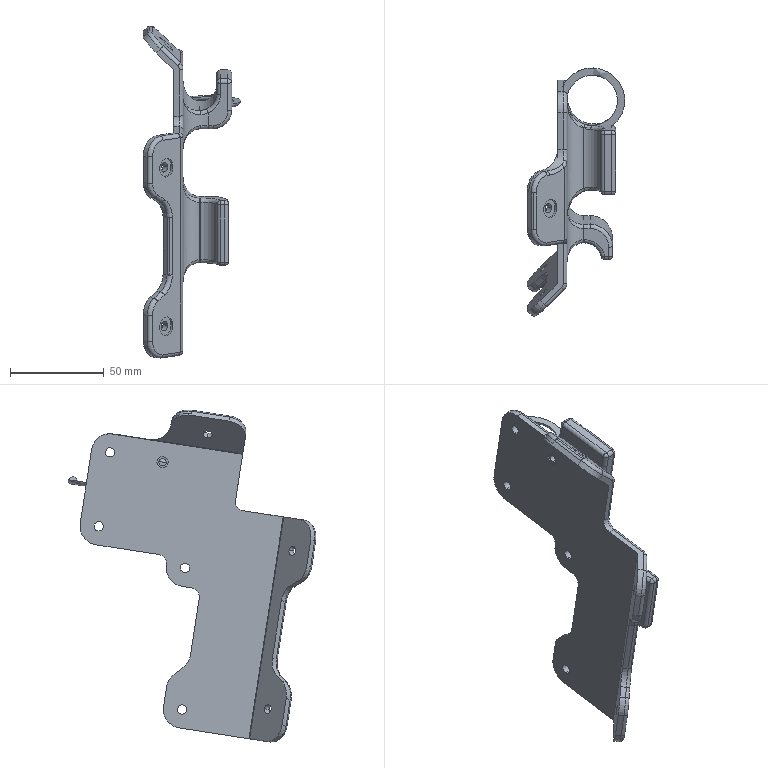Part | SolidWorks | features BaseBody 1 | 1 solid | 210 faces | box 52.213 x 132.591 x 177.573 mm | volume 88195 mm3 | cylinder 109 | plane 44 | torus 36 | spline 13 | sphere 8 | commonest cylinder face diameters 4 x45 10 x19 20 x16 5 x14 18 x8 1 x2